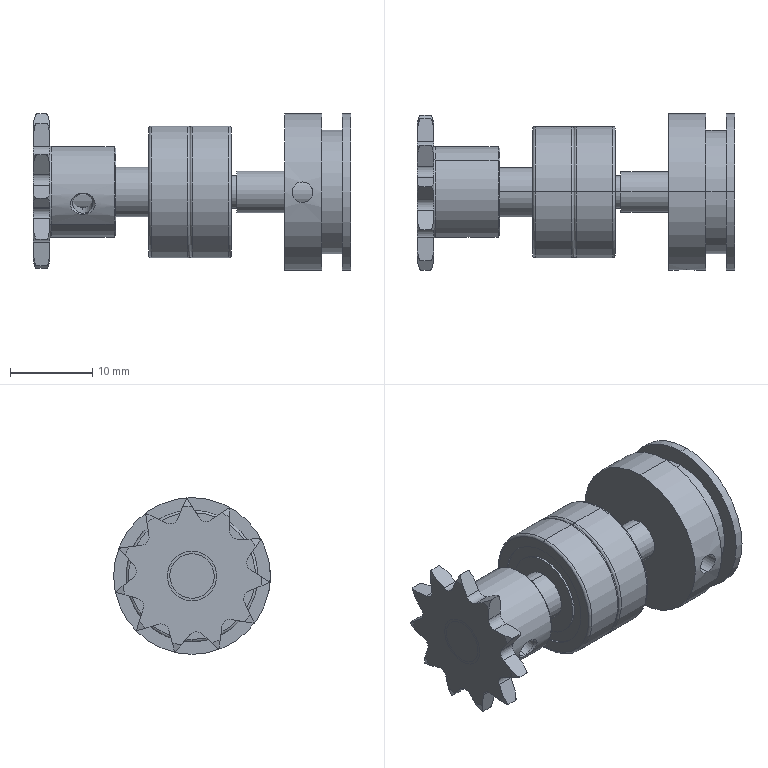Part | SolidWorks | 5 solids | 192 faces | box 38.5 x 19 x 19 mm | volume 5350 mm3 | cylinder 70 | plane 46 | torus 40 | cone 36 | commonest cylinder face diameters 2 x14 5 x12 10 x8 12.8 x8 3 x6 2.459 x4